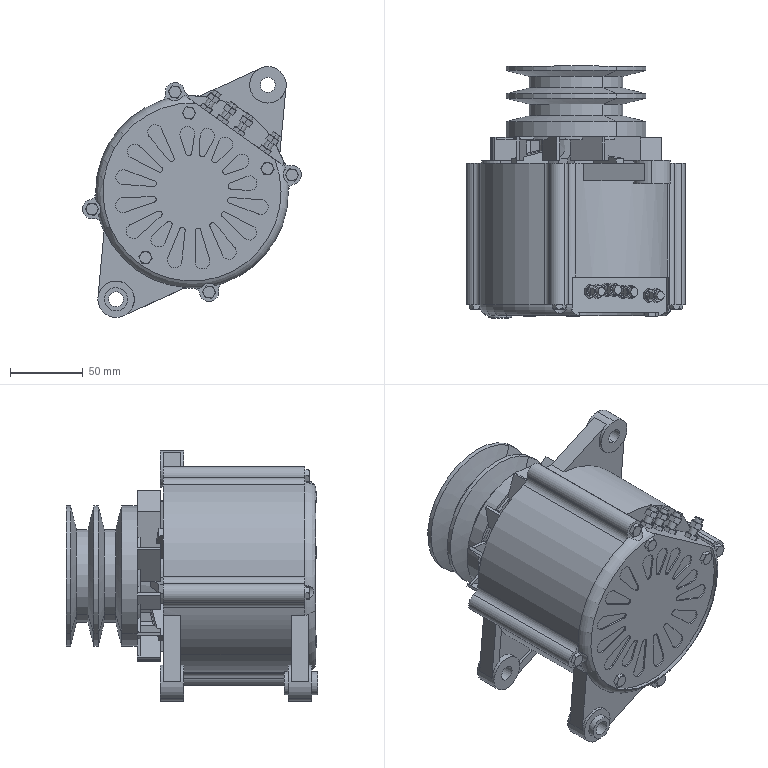Part | SolidWorks | features BaseBody 2 | 2 solids | 573 faces | box 150.011 x 172.427 x 171.911 mm | volume 1775646 mm3 | plane 314 | cylinder 143 | cone 115 | torus 1 | commonest cylinder face diameters 10 x47 4 x21 6 x16 92 x12 10.2 x6 12 x6